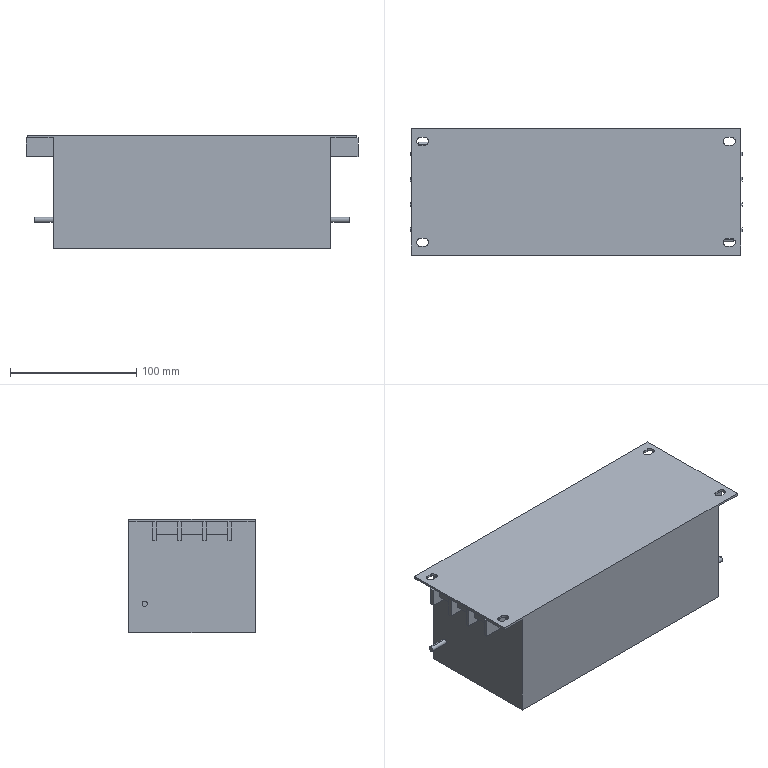Part | SolidWorks | features BaseBody 8 | 8 solids | 461 faces | box 263 x 100 x 90 mm | volume 2010436 mm3 | plane 342 | spline 91 | cylinder 28 | commonest cylinder face diameters 6 x12 6.4 x12 4 x4